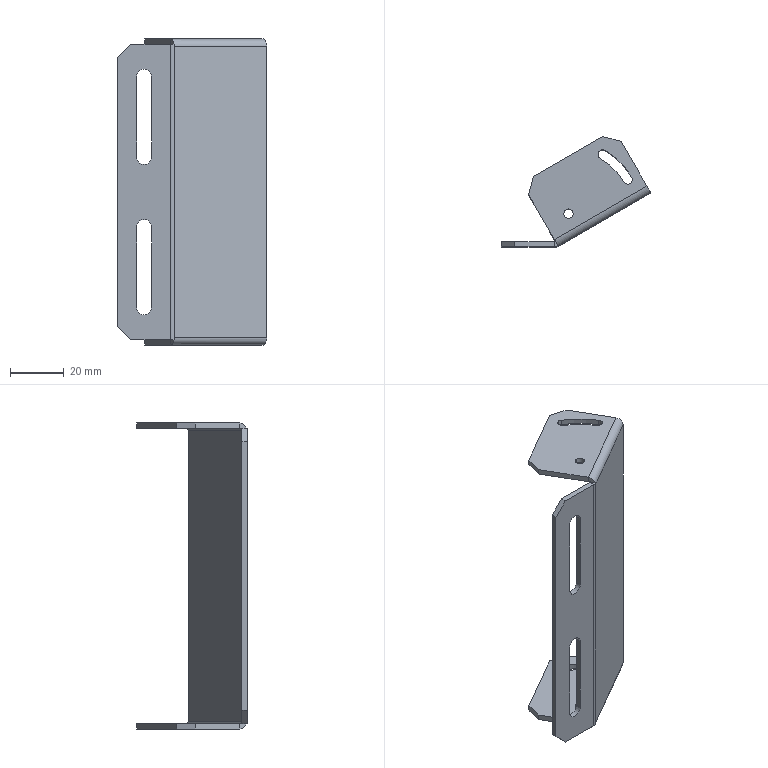Part | STEP file | CA-10-002Sensor Mounting Plate_Default | 1 solid | 60 faces | box 55.641 x 41.151 x 114 mm | volume 16325 mm3 | plane 36 | cylinder 24 | commonest cylinder face diameters 3.5 x10 5.5 x4 1.473 x3 5.473 x3 47.3 x2 54.3 x2